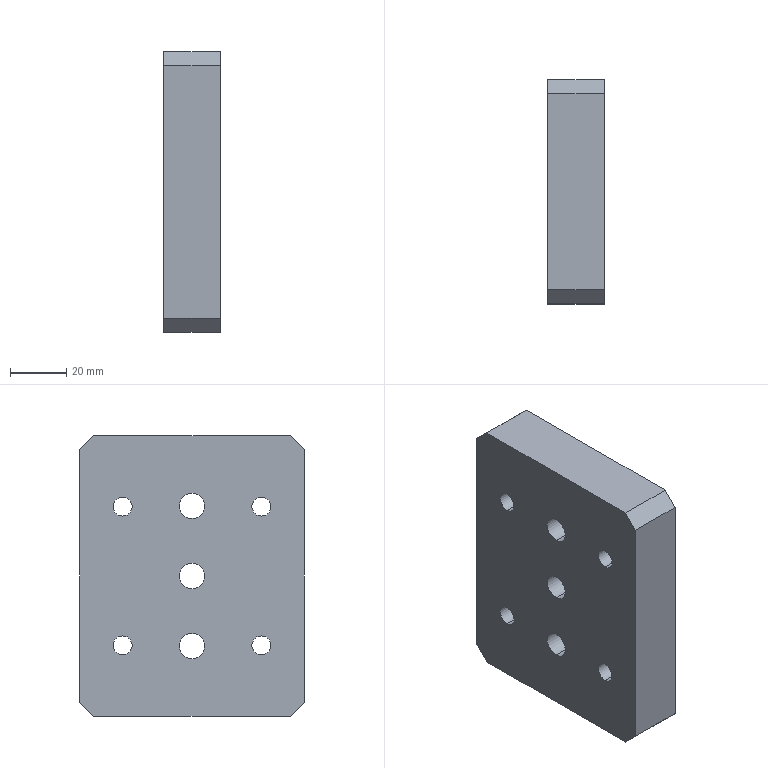Part | SolidWorks | features HoleWzd 2, Chamfer 1, Extrusion 1 | 1 solid | 33 faces | box 20 x 80 x 100 mm | volume 149224 mm3 | cylinder 20 | plane 13 | commonest cylinder face diameters 6.8 x8 9 x6 15 x6
STEP:
#1=CARTESIAN_POINT('',(11.,0.,32.5));
#2=VERTEX_POINT('',#1);
#3=CARTESIAN_POINT('',(11.,0.,17.5));
#4=VERTEX_POINT('',#3);
#5=CARTESIAN_POINT('',(11.,0.,25.));
#6=DIRECTION('',(1.,0.,0.));
#7=DIRECTION('',(0.,0.,-1.));
#8=AXIS2_PLACEMENT_3D('',#5,#6,#7);
#9=CIRCLE('',#8,7.5);
#10=EDGE_CURVE('',#2,#4,#9,.T.);
#11=ORIENTED_EDGE('',*,*,#10,.F.);
#12=CARTESIAN_POINT('',(20.,0.,32.5));
#13=VERTEX_POINT('',#12);
#14=CARTESIAN_POINT('',(20.,0.,32.5));
#15=DIRECTION('',(1.,0.,0.));
#16=VECTOR('',#15,1000.);
#17=LINE('',#14,#16);
#18=EDGE_CURVE('',#2,#13,#17,.T.);
#19=ORIENTED_EDGE('',*,*,#18,.T.);
#20=CARTESIAN_POINT('',(20.,0.,17.5));
#21=VERTEX_POINT('',#20);
#22=CARTESIAN_POINT('',(20.,0.,25.));
#23=DIRECTION('',(1.,0.,0.));
#24=DIRECTION('',(0.,0.,-1.));
#25=AXIS2_PLACEMENT_3D('',#22,#23,#24);
#26=CIRCLE('',#25,7.5);
#27=EDGE_CURVE('',#13,#21,#26,.T.);
#28=ORIENTED_EDGE('',*,*,#27,.T.);
#29=CARTESIAN_POINT('',(20.,0.,17.5));
#30=DIRECTION('',(1.,0.,0.));
#31=VECTOR('',#30,1000.);
#32=LINE('',#29,#31);
#33=EDGE_CURVE('',#4,#21,#32,.T.);
#34=ORIENTED_EDGE('',*,*,#33,.F.);
#35=EDGE_LOOP('',(#11,#19,#28,#34));
#36=FACE_OUTER_BOUND('',#35,.T.);
#37=CARTESIAN_POINT('',(20.,0.,25.));
#38=DIRECTION('',(1.,0.,0.));
#39=DIRECTION('',(0.,0.,-1.));
#40=AXIS2_PLACEMENT_3D('',#37,#38,#39);
#41=CYLINDRICAL_SURFACE('',#40,7.5);
#42=ADVANCED_FACE('',(#36),#41,.F.);
#43=CARTESIAN_POINT('',(0.,0.,29.5));
#44=VERTEX_POINT('',#43);
#45=CARTESIAN_POINT('',(0.,0.,20.5));
#46=VERTEX_POINT('',#45);
#47=CARTESIAN_POINT('',(0.,0.,25.));
#48=DIRECTION('',(1.,0.,0.));
#49=DIRECTION('',(0.,0.,-1.));
#50=AXIS2_PLACEMENT_3D('',#47,#48,#49);
#51=CIRCLE('',#50,4.5);
#52=EDGE_CURVE('',#44,#46,#51,.T.);
#53=ORIENTED_EDGE('',*,*,#52,.F.);
#54=CARTESIAN_POINT('',(11.,0.,29.5));
#55=VERTEX_POINT('',#54);
#56=CARTESIAN_POINT('',(20.,0.,29.5));
#57=DIRECTION('',(1.,0.,0.));
#58=VECTOR('',#57,1000.);
#59=LINE('',#56,#58);
#60=EDGE_CURVE('',#44,#55,#59,.T.);
#61=ORIENTED_EDGE('',*,*,#60,.T.);
#62=CARTESIAN_POINT('',(11.,0.,20.5));
#63=VERTEX_POINT('',#62);
#64=CARTESIAN_POINT('',(11.,0.,25.));
#65=DIRECTION('',(1.,0.,0.));
#66=DIRECTION('',(0.,0.,-1.));
#67=AXIS2_PLACEMENT_3D('',#64,#65,#66);
#68=CIRCLE('',#67,4.5);
#69=EDGE_CURVE('',#55,#63,#68,.T.);
#70=ORIENTED_EDGE('',*,*,#69,.T.);
#71=CARTESIAN_POINT('',(20.,0.,20.5));
#72=DIRECTION('',(1.,0.,0.));
#73=VECTOR('',#72,1000.);
#74=LINE('',#71,#73);
#75=EDGE_CURVE('',#46,#63,#74,.T.);
#76=ORIENTED_EDGE('',*,*,#75,.F.);
#77=EDGE_LOOP('',(#53,#61,#70,#76));
#78=FACE_OUTER_BOUND('',#77,.T.);
#79=CARTESIAN_POINT('',(20.,0.,25.));
#80=DIRECTION('',(1.,0.,0.));
#81=DIRECTION('',(0.,0.,-1.));
#82=AXIS2_PLACEMENT_3D('',#79,#80,#81);
#83=CYLINDRICAL_SURFACE('',#82,4.5);
#84=ADVANCED_FACE('',(#78),#83,.F.);
#85=CARTESIAN_POINT('',(11.,0.,7.5));
#86=VERTEX_POINT('',#85);
#87=CARTESIAN_POINT('',(11.,0.,-7.5));
#88=VERTEX_POINT('',#87);
#89=CARTESIAN_POINT('',(11.,0.,0.));
#90=DIRECTION('',(1.,0.,0.));
#91=DIRECTION('',(0.,0.,-1.));
#92=AXIS2_PLACEMENT_3D('',#89,#90,#91);
#93=CIRCLE('',#92,7.5);
#94=EDGE_CURVE('',#86,#88,#93,.T.);
#95=ORIENTED_EDGE('',*,*,#94,.F.);
#96=CARTESIAN_POINT('',(20.,0.,7.5));
#97=VERTEX_POINT('',#96);
#98=CARTESIAN_POINT('',(20.,0.,7.5));
#99=DIRECTION('',(1.,0.,0.));
#100=VECTOR('',#99,1000.);
#101=LINE('',#98,#100);
#102=EDGE_CURVE('',#86,#97,#101,.T.);
#103=ORIENTED_EDGE('',*,*,#102,.T.);
#104=CARTESIAN_POINT('',(20.,0.,-7.5));
#105=VERTEX_POINT('',#104);
#106=CARTESIAN_POINT('',(20.,0.,0.));
#107=DIRECTION('',(1.,0.,0.));
#108=DIRECTION('',(0.,0.,-1.));
#109=AXIS2_PLACEMENT_3D('',#106,#107,#108);
#110=CIRCLE('',#109,7.5);
#111=EDGE_CURVE('',#97,#105,#110,.T.);
#112=ORIENTED_EDGE('',*,*,#111,.T.);
#113=CARTESIAN_POINT('',(20.,0.,-7.5));
#114=DIRECTION('',(1.,0.,0.));
#115=VECTOR('',#114,1000.);
#116=LINE('',#113,#115);
#117=EDGE_CURVE('',#88,#105,#116,.T.);
#118=ORIENTED_EDGE('',*,*,#117,.F.);
#119=EDGE_LOOP('',(#95,#103,#112,#118));
#120=FACE_OUTER_BOUND('',#119,.T.);
#121=CARTESIAN_POINT('',(20.,0.,0.));
#122=DIRECTION('',(1.,0.,0.));
#123=DIRECTION('',(0.,0.,-1.));
#124=AXIS2_PLACEMENT_3D('',#121,#122,#123);
#125=CYLINDRICAL_SURFACE('',#124,7.5);
#126=ADVANCED_FACE('',(#120),#125,.F.);
#127=CARTESIAN_POINT('',(0.,0.,4.5));
#128=VERTEX_POINT('',#127);
#129=CARTESIAN_POINT('',(0.,0.,-4.5));
#130=VERTEX_POINT('',#129);
#131=CARTESIAN_POINT('',(0.,0.,0.));
#132=DIRECTION('',(1.,0.,0.));
#133=DIRECTION('',(0.,0.,-1.));
#134=AXIS2_PLACEMENT_3D('',#131,#132,#133);
#135=CIRCLE('',#134,4.5);
#136=EDGE_CURVE('',#128,#130,#135,.T.);
#137=ORIENTED_EDGE('',*,*,#136,.F.);
#138=CARTESIAN_POINT('',(11.,0.,4.5));
#139=VERTEX_POINT('',#138);
#140=CARTESIAN_POINT('',(20.,0.,4.5));
#141=DIRECTION('',(1.,0.,0.));
#142=VECTOR('',#141,1000.);
#143=LINE('',#140,#142);
#144=EDGE_CURVE('',#128,#139,#143,.T.);
#145=ORIENTED_EDGE('',*,*,#144,.T.);
#146=CARTESIAN_POINT('',(11.,0.,-4.5));
#147=VERTEX_POINT('',#146);
#148=CARTESIAN_POINT('',(11.,0.,0.));
#149=DIRECTION('',(1.,0.,0.));
#150=DIRECTION('',(0.,0.,-1.));
#151=AXIS2_PLACEMENT_3D('',#148,#149,#150);
#152=CIRCLE('',#151,4.5);
#153=EDGE_CURVE('',#139,#147,#152,.T.);
#154=ORIENTED_EDGE('',*,*,#153,.T.);
#155=CARTESIAN_POINT('',(20.,0.,-4.5));
#156=DIRECTION('',(1.,0.,0.));
#157=VECTOR('',#156,1000.);
#158=LINE('',#155,#157);
#159=EDGE_CURVE('',#130,#147,#158,.T.);
#160=ORIENTED_EDGE('',*,*,#159,.F.);
#161=EDGE_LOOP('',(#137,#145,#154,#160));
#162=FACE_OUTER_BOUND('',#161,.T.);
#163=CARTESIAN_POINT('',(20.,0.,0.));
#164=DIRECTION('',(1.,0.,0.));
#165=DIRECTION('',(0.,0.,-1.));
#166=AXIS2_PLACEMENT_3D('',#163,#164,#165);
#167=CYLINDRICAL_SURFACE('',#166,4.5);
#168=ADVANCED_FACE('',(#162),#167,.F.);
#169=CARTESIAN_POINT('',(11.,0.,-17.5));
#170=VERTEX_POINT('',#169);
#171=CARTESIAN_POINT('',(11.,0.,-32.5));
#172=VERTEX_POINT('',#171);
#173=CARTESIAN_POINT('',(11.,0.,-25.));
#174=DIRECTION('',(1.,0.,0.));
#175=DIRECTION('',(0.,0.,-1.));
#176=AXIS2_PLACEMENT_3D('',#173,#174,#175);
#177=CIRCLE('',#176,7.5);
#178=EDGE_CURVE('',#170,#172,#177,.T.);
#179=ORIENTED_EDGE('',*,*,#178,.F.);
#180=CARTESIAN_POINT('',(20.,0.,-17.5));
#181=VERTEX_POINT('',#180);
#182=CARTESIAN_POINT('',(20.,0.,-17.5));
#183=DIRECTION('',(1.,0.,0.));
#184=VECTOR('',#183,1000.);
#185=LINE('',#182,#184);
#186=EDGE_CURVE('',#170,#181,#185,.T.);
#187=ORIENTED_EDGE('',*,*,#186,.T.);
#188=CARTESIAN_POINT('',(20.,0.,-32.5));
#189=VERTEX_POINT('',#188);
#190=CARTESIAN_POINT('',(20.,0.,-25.));
#191=DIRECTION('',(1.,0.,0.));
#192=DIRECTION('',(0.,0.,-1.));
#193=AXIS2_PLACEMENT_3D('',#190,#191,#192);
#194=CIRCLE('',#193,7.5);
#195=EDGE_CURVE('',#181,#189,#194,.T.);
#196=ORIENTED_EDGE('',*,*,#195,.T.);
#197=CARTESIAN_POINT('',(20.,0.,-32.5));
#198=DIRECTION('',(1.,0.,0.));
#199=VECTOR('',#198,1000.);
#200=LINE('',#197,#199);
#201=EDGE_CURVE('',#172,#189,#200,.T.);
#202=ORIENTED_EDGE('',*,*,#201,.F.);
#203=EDGE_LOOP('',(#179,#187,#196,#202));
#204=FACE_OUTER_BOUND('',#203,.T.);
#205=CARTESIAN_POINT('',(20.,0.,-25.));
#206=DIRECTION('',(1.,0.,0.));
#207=DIRECTION('',(0.,0.,-1.));
#208=AXIS2_PLACEMENT_3D('',#205,#206,#207);
#209=CYLINDRICAL_SURFACE('',#208,7.5);
#210=ADVANCED_FACE('',(#204),#209,.F.);
#211=CARTESIAN_POINT('',(0.,0.,-20.5));
#212=VERTEX_POINT('',#211);
#213=CARTESIAN_POINT('',(0.,0.,-29.5));
#214=VERTEX_POINT('',#213);
#215=CARTESIAN_POINT('',(0.,0.,-25.));
#216=DIRECTION('',(1.,0.,0.));
#217=DIRECTION('',(0.,0.,-1.));
#218=AXIS2_PLACEMENT_3D('',#215,#216,#217);
#219=CIRCLE('',#218,4.5);
#220=EDGE_CURVE('',#212,#214,#219,.T.);
#221=ORIENTED_EDGE('',*,*,#220,.F.);
#222=CARTESIAN_POINT('',(11.,0.,-20.5));
#223=VERTEX_POINT('',#222);
#224=CARTESIAN_POINT('',(20.,0.,-20.5));
#225=DIRECTION('',(1.,0.,0.));
#226=VECTOR('',#225,1000.);
#227=LINE('',#224,#226);
#228=EDGE_CURVE('',#212,#223,#227,.T.);
#229=ORIENTED_EDGE('',*,*,#228,.T.);
#230=CARTESIAN_POINT('',(11.,0.,-29.5));
#231=VERTEX_POINT('',#230);
#232=CARTESIAN_POINT('',(11.,0.,-25.));
#233=DIRECTION('',(1.,0.,0.));
#234=DIRECTION('',(0.,0.,-1.));
#235=AXIS2_PLACEMENT_3D('',#232,#233,#234);
#236=CIRCLE('',#235,4.5);
#237=EDGE_CURVE('',#223,#231,#236,.T.);
#238=ORIENTED_EDGE('',*,*,#237,.T.);
#239=CARTESIAN_POINT('',(20.,0.,-29.5));
#240=DIRECTION('',(1.,0.,0.));
#241=VECTOR('',#240,1000.);
#242=LINE('',#239,#241);
#243=EDGE_CURVE('',#214,#231,#242,.T.);
#244=ORIENTED_EDGE('',*,*,#243,.F.);
#245=EDGE_LOOP('',(#221,#229,#238,#244));
#246=FACE_OUTER_BOUND('',#245,.T.);
#247=CARTESIAN_POINT('',(20.,0.,-25.));
#248=DIRECTION('',(1.,0.,0.));
#249=DIRECTION('',(0.,0.,-1.));
#250=AXIS2_PLACEMENT_3D('',#247,#248,#249);
#251=CYLINDRICAL_SURFACE('',#250,4.5);
#252=ADVANCED_FACE('',(#246),#251,.F.);
#253=CARTESIAN_POINT('',(0.,24.749,28.149));
#254=VERTEX_POINT('',#253);
#255=CARTESIAN_POINT('',(0.,24.749,21.349));
#256=VERTEX_POINT('',#255);
#257=CARTESIAN_POINT('',(0.,24.749,24.749));
#258=DIRECTION('',(1.,0.,0.));
#259=DIRECTION('',(0.,0.,-1.));
#260=AXIS2_PLACEMENT_3D('',#257,#258,#259);
#261=CIRCLE('',#260,3.4);
#262=EDGE_CURVE('',#254,#256,#261,.T.);
#263=ORIENTED_EDGE('',*,*,#262,.F.);
#264=CARTESIAN_POINT('',(20.,24.749,28.149));
#265=VERTEX_POINT('',#264);
#266=CARTESIAN_POINT('',(20.,24.749,28.149));
#267=DIRECTION('',(1.,0.,0.));
#268=VECTOR('',#267,1000.);
#269=LINE('',#266,#268);
#270=EDGE_CURVE('',#254,#265,#269,.T.);
#271=ORIENTED_EDGE('',*,*,#270,.T.);
#272=CARTESIAN_POINT('',(20.,24.749,21.349));
#273=VERTEX_POINT('',#272);
#274=CARTESIAN_POINT('',(20.,24.749,24.749));
#275=DIRECTION('',(1.,0.,0.));
#276=DIRECTION('',(0.,0.,-1.));
#277=AXIS2_PLACEMENT_3D('',#274,#275,#276);
#278=CIRCLE('',#277,3.4);
#279=EDGE_CURVE('',#265,#273,#278,.T.);
#280=ORIENTED_EDGE('',*,*,#279,.T.);
#281=CARTESIAN_POINT('',(20.,24.749,21.349));
#282=DIRECTION('',(1.,0.,0.));
#283=VECTOR('',#282,1000.);
#284=LINE('',#281,#283);
#285=EDGE_CURVE('',#256,#273,#284,.T.);
#286=ORIENTED_EDGE('',*,*,#285,.F.);
#287=EDGE_LOOP('',(#263,#271,#280,#286));
#288=FACE_OUTER_BOUND('',#287,.T.);
#289=CARTESIAN_POINT('',(20.,24.749,24.749));
#290=DIRECTION('',(1.,0.,0.));
#291=DIRECTION('',(0.,0.,-1.));
#292=AXIS2_PLACEMENT_3D('',#289,#290,#291);
#293=CYLINDRICAL_SURFACE('',#292,3.4);
#294=ADVANCED_FACE('',(#288),#293,.F.);
#295=CARTESIAN_POINT('',(0.,24.749,-21.349));
#296=VERTEX_POINT('',#295);
#297=CARTESIAN_POINT('',(0.,24.749,-28.149));
#298=VERTEX_POINT('',#297);
#299=CARTESIAN_POINT('',(0.,24.749,-24.749));
#300=DIRECTION('',(1.,0.,0.));
#301=DIRECTION('',(0.,0.,-1.));
#302=AXIS2_PLACEMENT_3D('',#299,#300,#301);
#303=CIRCLE('',#302,3.4);
#304=EDGE_CURVE('',#296,#298,#303,.T.);
#305=ORIENTED_EDGE('',*,*,#304,.F.);
#306=CARTESIAN_POINT('',(20.,24.749,-21.349));
#307=VERTEX_POINT('',#306);
#308=CARTESIAN_POINT('',(20.,24.749,-21.349));
#309=DIRECTION('',(1.,0.,0.));
#310=VECTOR('',#309,1000.);
#311=LINE('',#308,#310);
#312=EDGE_CURVE('',#296,#307,#311,.T.);
#313=ORIENTED_EDGE('',*,*,#312,.T.);
#314=CARTESIAN_POINT('',(20.,24.749,-28.149));
#315=VERTEX_POINT('',#314);
#316=CARTESIAN_POINT('',(20.,24.749,-24.749));
#317=DIRECTION('',(1.,0.,0.));
#318=DIRECTION('',(0.,0.,-1.));
#319=AXIS2_PLACEMENT_3D('',#316,#317,#318);
#320=CIRCLE('',#319,3.4);
#321=EDGE_CURVE('',#307,#315,#320,.T.);
#322=ORIENTED_EDGE('',*,*,#321,.T.);
#323=CARTESIAN_POINT('',(20.,24.749,-28.149));
#324=DIRECTION('',(1.,0.,0.));
#325=VECTOR('',#324,1000.);
#326=LINE('',#323,#325);
#327=EDGE_CURVE('',#298,#315,#326,.T.);
#328=ORIENTED_EDGE('',*,*,#327,.F.);
#329=EDGE_LOOP('',(#305,#313,#322,#328));
#330=FACE_OUTER_BOUND('',#329,.T.);
#331=CARTESIAN_POINT('',(20.,24.749,-24.749));
#332=DIRECTION('',(1.,0.,0.));
#333=DIRECTION('',(0.,0.,-1.));
#334=AXIS2_PLACEMENT_3D('',#331,#332,#333);
#335=CYLINDRICAL_SURFACE('',#334,3.4);
#336=ADVANCED_FACE('',(#330),#335,.F.);
#337=CARTESIAN_POINT('',(0.,-24.749,-21.349));
#338=VERTEX_POINT('',#337);
#339=CARTESIAN_POINT('',(0.,-24.749,-28.149));
#340=VERTEX_POINT('',#339);
#341=CARTESIAN_POINT('',(0.,-24.749,-24.749));
#342=DIRECTION('',(1.,0.,0.));
#343=DIRECTION('',(0.,0.,-1.));
#344=AXIS2_PLACEMENT_3D('',#341,#342,#343);
#345=CIRCLE('',#344,3.4);
#346=EDGE_CURVE('',#338,#340,#345,.T.);
#347=ORIENTED_EDGE('',*,*,#346,.F.);
#348=CARTESIAN_POINT('',(20.,-24.749,-21.349));
#349=VERTEX_POINT('',#348);
#350=CARTESIAN_POINT('',(20.,-24.749,-21.349));
#351=DIRECTION('',(1.,0.,0.));
#352=VECTOR('',#351,1000.);
#353=LINE('',#350,#352);
#354=EDGE_CURVE('',#338,#349,#353,.T.);
#355=ORIENTED_EDGE('',*,*,#354,.T.);
#356=CARTESIAN_POINT('',(20.,-24.749,-28.149));
#357=VERTEX_POINT('',#356);
#358=CARTESIAN_POINT('',(20.,-24.749,-24.749));
#359=DIRECTION('',(1.,0.,0.));
#360=DIRECTION('',(0.,0.,-1.));
#361=AXIS2_PLACEMENT_3D('',#358,#359,#360);
#362=CIRCLE('',#361,3.4);
#363=EDGE_CURVE('',#349,#357,#362,.T.);
#364=ORIENTED_EDGE('',*,*,#363,.T.);
#365=CARTESIAN_POINT('',(20.,-24.749,-28.149));
#366=DIRECTION('',(1.,0.,0.));
#367=VECTOR('',#366,1000.);
#368=LINE('',#365,#367);
#369=EDGE_CURVE('',#340,#357,#368,.T.);
#370=ORIENTED_EDGE('',*,*,#369,.F.);
#371=EDGE_LOOP('',(#347,#355,#364,#370));
#372=FACE_OUTER_BOUND('',#371,.T.);
#373=CARTESIAN_POINT('',(20.,-24.749,-24.749));
#374=DIRECTION('',(1.,0.,0.));
#375=DIRECTION('',(0.,0.,-1.));
#376=AXIS2_PLACEMENT_3D('',#373,#374,#375);
#377=CYLINDRICAL_SURFACE('',#376,3.4);
#378=ADVANCED_FACE('',(#372),#377,.F.);
#379=CARTESIAN_POINT('',(0.,-24.749,28.149));
#380=VERTEX_POINT('',#379);
#381=CARTESIAN_POINT('',(0.,-24.749,21.349));
#382=VERTEX_POINT('',#381);
#383=CARTESIAN_POINT('',(0.,-24.749,24.749));
#384=DIRECTION('',(1.,0.,0.));
#385=DIRECTION('',(0.,0.,-1.));
#386=AXIS2_PLACEMENT_3D('',#383,#384,#385);
#387=CIRCLE('',#386,3.4);
#388=EDGE_CURVE('',#380,#382,#387,.T.);
#389=ORIENTED_EDGE('',*,*,#388,.F.);
#390=CARTESIAN_POINT('',(20.,-24.749,28.149));
#391=VERTEX_POINT('',#390);
#392=CARTESIAN_POINT('',(20.,-24.749,28.149));
#393=DIRECTION('',(1.,0.,0.));
#394=VECTOR('',#393,1000.);
#395=LINE('',#392,#394);
#396=EDGE_CURVE('',#380,#391,#395,.T.);
#397=ORIENTED_EDGE('',*,*,#396,.T.);
#398=CARTESIAN_POINT('',(20.,-24.749,21.349));
#399=VERTEX_POINT('',#398);
#400=CARTESIAN_POINT('',(20.,-24.749,24.749));
#401=DIRECTION('',(1.,0.,0.));
#402=DIRECTION('',(0.,0.,-1.));
#403=AXIS2_PLACEMENT_3D('',#400,#401,#402);
#404=CIRCLE('',#403,3.4);
#405=EDGE_CURVE('',#391,#399,#404,.T.);
#406=ORIENTED_EDGE('',*,*,#405,.T.);
#407=CARTESIAN_POINT('',(20.,-24.749,21.349));
#408=DIRECTION('',(1.,0.,0.));
#409=VECTOR('',#408,1000.);
#410=LINE('',#407,#409);
#411=EDGE_CURVE('',#382,#399,#410,.T.);
#412=ORIENTED_EDGE('',*,*,#411,.F.);
#413=EDGE_LOOP('',(#389,#397,#406,#412));
#414=FACE_OUTER_BOUND('',#413,.T.);
#415=CARTESIAN_POINT('',(20.,-24.749,24.749));
#416=DIRECTION('',(1.,0.,0.));
#417=DIRECTION('',(0.,0.,-1.));
#418=AXIS2_PLACEMENT_3D('',#415,#416,#417);
#419=CYLINDRICAL_SURFACE('',#418,3.4);
#420=ADVANCED_FACE('',(#414),#419,.F.);
#421=CARTESIAN_POINT('',(0.,-35.,-50.));
#422=VERTEX_POINT('',#421);
#423=CARTESIAN_POINT('',(0.,35.,-50.));
#424=VERTEX_POINT('',#423);
#425=CARTESIAN_POINT('',(0.,40.,-50.));
#426=DIRECTION('',(0.,1.,0.));
#427=VECTOR('',#426,1000.);
#428=LINE('',#425,#427);
#429=EDGE_CURVE('',#422,#424,#428,.T.);
#430=ORIENTED_EDGE('',*,*,#429,.T.);
#431=CARTESIAN_POINT('',(20.,35.,-50.));
#432=VERTEX_POINT('',#431);
#433=CARTESIAN_POINT('',(20.,35.,-50.));
#434=DIRECTION('',(1.,0.,0.));
#435=VECTOR('',#434,1000.);
#436=LINE('',#433,#435);
#437=EDGE_CURVE('',#424,#432,#436,.T.);
#438=ORIENTED_EDGE('',*,*,#437,.T.);
#439=CARTESIAN_POINT('',(20.,-35.,-50.));
#440=VERTEX_POINT('',#439);
#441=CARTESIAN_POINT('',(20.,40.,-50.));
#442=DIRECTION('',(0.,1.,0.));
#443=VECTOR('',#442,1000.);
#444=LINE('',#441,#443);
#445=EDGE_CURVE('',#440,#432,#444,.T.);
#446=ORIENTED_EDGE('',*,*,#445,.F.);
#447=CARTESIAN_POINT('',(20.,-35.,-50.));
#448=DIRECTION('',(-1.,0.,0.));
#449=VECTOR('',#448,1000.);
#450=LINE('',#447,#449);
#451=EDGE_CURVE('',#440,#422,#450,.T.);
#452=ORIENTED_EDGE('',*,*,#451,.T.);
#453=EDGE_LOOP('',(#430,#438,#446,#452));
#454=FACE_OUTER_BOUND('',#453,.T.);
#455=CARTESIAN_POINT('',(20.,40.,-50.));
#456=DIRECTION('',(0.,0.,1.));
#457=DIRECTION('',(0.,-1.,0.));
#458=AXIS2_PLACEMENT_3D('',#455,#456,#457);
#459=PLANE('',#458);
#460=ADVANCED_FACE('',(#454),#459,.F.);
#461=CARTESIAN_POINT('',(20.,40.,-45.));
#462=VERTEX_POINT('',#461);
#463=CARTESIAN_POINT('',(20.,40.,45.));
#464=VERTEX_POINT('',#463);
#465=CARTESIAN_POINT('',(20.,40.,50.));
#466=DIRECTION('',(0.,0.,1.));
#467=VECTOR('',#466,1000.);
#468=LINE('',#465,#467);
#469=EDGE_CURVE('',#462,#464,#468,.T.);
#470=ORIENTED_EDGE('',*,*,#469,.F.);
#471=CARTESIAN_POINT('',(0.,40.,-45.));
#472=VERTEX_POINT('',#471);
#473=CARTESIAN_POINT('',(20.,40.,-45.));
#474=DIRECTION('',(-1.,0.,0.));
#475=VECTOR('',#474,1000.);
#476=LINE('',#473,#475);
#477=EDGE_CURVE('',#462,#472,#476,.T.);
#478=ORIENTED_EDGE('',*,*,#477,.T.);
#479=CARTESIAN_POINT('',(0.,40.,45.));
#480=VERTEX_POINT('',#479);
#481=CARTESIAN_POINT('',(0.,40.,50.));
#482=DIRECTION('',(0.,0.,1.));
#483=VECTOR('',#482,1000.);
#484=LINE('',#481,#483);
#485=EDGE_CURVE('',#472,#480,#484,.T.);
#486=ORIENTED_EDGE('',*,*,#485,.T.);
#487=CARTESIAN_POINT('',(20.,40.,45.));
#488=DIRECTION('',(1.,0.,0.));
#489=VECTOR('',#488,1000.);
#490=LINE('',#487,#489);
#491=EDGE_CURVE('',#480,#464,#490,.T.);
#492=ORIENTED_EDGE('',*,*,#491,.T.);
#493=EDGE_LOOP('',(#470,#478,#486,#492));
#494=FACE_OUTER_BOUND('',#493,.T.);
#495=CARTESIAN_POINT('',(20.,40.,50.));
#496=DIRECTION('',(0.,-1.,0.));
#497=DIRECTION('',(0.,0.,-1.));
#498=AXIS2_PLACEMENT_3D('',#495,#496,#497);
#499=PLANE('',#498);
#500=ADVANCED_FACE('',(#494),#499,.F.);
#501=CARTESIAN_POINT('',(20.,35.,50.));
#502=VERTEX_POINT('',#501);
#503=CARTESIAN_POINT('',(20.,-35.,50.));
#504=VERTEX_POINT('',#503);
#505=CARTESIAN_POINT('',(20.,40.,50.));
#506=DIRECTION('',(0.,-1.,0.));
#507=VECTOR('',#506,1000.);
#508=LINE('',#505,#507);
#509=EDGE_CURVE('',#502,#504,#508,.T.);
#510=ORIENTED_EDGE('',*,*,#509,.F.);
#511=CARTESIAN_POINT('',(0.,35.,50.));
#512=VERTEX_POINT('',#511);
#513=CARTESIAN_POINT('',(20.,35.,50.));
#514=DIRECTION('',(-1.,0.,0.));
#515=VECTOR('',#514,1000.);
#516=LINE('',#513,#515);
#517=EDGE_CURVE('',#502,#512,#516,.T.);
#518=ORIENTED_EDGE('',*,*,#517,.T.);
#519=CARTESIAN_POINT('',(0.,-35.,50.));
#520=VERTEX_POINT('',#519);
#521=CARTESIAN_POINT('',(0.,40.,50.));
#522=DIRECTION('',(0.,-1.,0.));
#523=VECTOR('',#522,1000.);
#524=LINE('',#521,#523);
#525=EDGE_CURVE('',#512,#520,#524,.T.);
#526=ORIENTED_EDGE('',*,*,#525,.T.);
#527=CARTESIAN_POINT('',(20.,-35.,50.));
#528=DIRECTION('',(1.,0.,0.));
#529=VECTOR('',#528,1000.);
#530=LINE('',#527,#529);
#531=EDGE_CURVE('',#520,#504,#530,.T.);
#532=ORIENTED_EDGE('',*,*,#531,.T.);
#533=EDGE_LOOP('',(#510,#518,#526,#532));
#534=FACE_OUTER_BOUND('',#533,.T.);
#535=CARTESIAN_POINT('',(20.,40.,50.));
#536=DIRECTION('',(0.,0.,-1.));
#537=DIRECTION('',(0.,1.,0.));
#538=AXIS2_PLACEMENT_3D('',#535,#536,#537);
#539=PLANE('',#538);
#540=ADVANCED_FACE('',(#534),#539,.F.);
#541=CARTESIAN_POINT('',(0.,-40.,45.));
#542=VERTEX_POINT('',#541);
#543=CARTESIAN_POINT('',(0.,-40.,-45.));
#544=VERTEX_POINT('',#543);
#545=CARTESIAN_POINT('',(0.,-40.,50.));
#546=DIRECTION('',(0.,0.,-1.));
#547=VECTOR('',#546,1000.);
#548=LINE('',#545,#547);
#549=EDGE_CURVE('',#542,#544,#548,.T.);
#550=ORIENTED_EDGE('',*,*,#549,.T.);
#551=CARTESIAN_POINT('',(20.,-40.,-45.));
#552=VERTEX_POINT('',#551);
#553=CARTESIAN_POINT('',(20.,-40.,-45.));
#554=DIRECTION('',(1.,0.,0.));
#555=VECTOR('',#554,1000.);
#556=LINE('',#553,#555);
#557=EDGE_CURVE('',#544,#552,#556,.T.);
#558=ORIENTED_EDGE('',*,*,#557,.T.);
#559=CARTESIAN_POINT('',(20.,-40.,45.));
#560=VERTEX_POINT('',#559);
#561=CARTESIAN_POINT('',(20.,-40.,50.));
#562=DIRECTION('',(0.,0.,-1.));
#563=VECTOR('',#562,1000.);
#564=LINE('',#561,#563);
#565=EDGE_CURVE('',#560,#552,#564,.T.);
#566=ORIENTED_EDGE('',*,*,#565,.F.);
#567=CARTESIAN_POINT('',(20.,-40.,45.));
#568=DIRECTION('',(-1.,0.,0.));
#569=VECTOR('',#568,1000.);
#570=LINE('',#567,#569);
#571=EDGE_CURVE('',#560,#542,#570,.T.);
#572=ORIENTED_EDGE('',*,*,#571,.T.);
#573=EDGE_LOOP('',(#550,#558,#566,#572));
#574=FACE_OUTER_BOUND('',#573,.T.);
#575=CARTESIAN_POINT('',(20.,-40.,50.));
#576=DIRECTION('',(0.,1.,0.));
#577=DIRECTION('',(0.,0.,1.));
#578=AXIS2_PLACEMENT_3D('',#575,#576,#577);
#579=PLANE('',#578);
#580=ADVANCED_FACE('',(#574),#579,.F.);
#581=CARTESIAN_POINT('',(20.,0.,25.));
#582=DIRECTION('',(1.,0.,0.));
#583=DIRECTION('',(0.,0.,-1.));
#584=AXIS2_PLACEMENT_3D('',#581,#582,#583);
#585=CIRCLE('',#584,7.5);
#586=EDGE_CURVE('',#21,#13,#585,.T.);
#587=ORIENTED_EDGE('',*,*,#586,.F.);
#588=ORIENTED_EDGE('',*,*,#27,.F.);
#589=EDGE_LOOP('',(#587,#588));
#590=FACE_BOUND('',#589,.T.);
#591=CARTESIAN_POINT('',(20.,0.,0.));
#592=DIRECTION('',(1.,0.,0.));
#593=DIRECTION('',(0.,0.,-1.));
#594=AXIS2_PLACEMENT_3D('',#591,#592,#593);
#595=CIRCLE('',#594,7.5);
#596=EDGE_CURVE('',#105,#97,#595,.T.);
#597=ORIENTED_EDGE('',*,*,#596,.F.);
#598=ORIENTED_EDGE('',*,*,#111,.F.);
#599=EDGE_LOOP('',(#597,#598));
#600=FACE_BOUND('',#599,.T.);
#601=CARTESIAN_POINT('',(20.,0.,-25.));
#602=DIRECTION('',(1.,0.,0.));
#603=DIRECTION('',(0.,0.,-1.));
#604=AXIS2_PLACEMENT_3D('',#601,#602,#603);
#605=CIRCLE('',#604,7.5);
#606=EDGE_CURVE('',#189,#181,#605,.T.);
#607=ORIENTED_EDGE('',*,*,#606,.F.);
#608=ORIENTED_EDGE('',*,*,#195,.F.);
#609=EDGE_LOOP('',(#607,#608));
#610=FACE_BOUND('',#609,.T.);
#611=CARTESIAN_POINT('',(20.,24.749,24.749));
#612=DIRECTION('',(1.,0.,0.));
#613=DIRECTION('',(0.,0.,-1.));
#614=AXIS2_PLACEMENT_3D('',#611,#612,#613);
#615=CIRCLE('',#614,3.4);
#616=EDGE_CURVE('',#273,#265,#615,.T.);
#617=ORIENTED_EDGE('',*,*,#616,.F.);
#618=ORIENTED_EDGE('',*,*,#279,.F.);
#619=EDGE_LOOP('',(#617,#618));
#620=FACE_BOUND('',#619,.T.);
#621=CARTESIAN_POINT('',(20.,24.749,-24.749));
#622=DIRECTION('',(1.,0.,0.));
#623=DIRECTION('',(0.,0.,-1.));
#624=AXIS2_PLACEMENT_3D('',#621,#622,#623);
#625=CIRCLE('',#624,3.4);
#626=EDGE_CURVE('',#315,#307,#625,.T.);
#627=ORIENTED_EDGE('',*,*,#626,.F.);
#628=ORIENTED_EDGE('',*,*,#321,.F.);
#629=EDGE_LOOP('',(#627,#628));
#630=FACE_BOUND('',#629,.T.);
#631=CARTESIAN_POINT('',(20.,-24.749,-24.749));
#632=DIRECTION('',(1.,0.,0.));
#633=DIRECTION('',(0.,0.,-1.));
#634=AXIS2_PLACEMENT_3D('',#631,#632,#633);
#635=CIRCLE('',#634,3.4);
#636=EDGE_CURVE('',#357,#349,#635,.T.);
#637=ORIENTED_EDGE('',*,*,#636,.F.);
#638=ORIENTED_EDGE('',*,*,#363,.F.);
#639=EDGE_LOOP('',(#637,#638));
#640=FACE_BOUND('',#639,.T.);
#641=CARTESIAN_POINT('',(20.,-24.749,24.749));
#642=DIRECTION('',(1.,0.,0.));
#643=DIRECTION('',(0.,0.,-1.));
#644=AXIS2_PLACEMENT_3D('',#641,#642,#643);
#645=CIRCLE('',#644,3.4);
#646=EDGE_CURVE('',#399,#391,#645,.T.);
#647=ORIENTED_EDGE('',*,*,#646,.F.);
#648=ORIENTED_EDGE('',*,*,#405,.F.);
#649=EDGE_LOOP('',(#647,#648));
#650=FACE_BOUND('',#649,.T.);
#651=ORIENTED_EDGE('',*,*,#445,.T.);
#652=CARTESIAN_POINT('',(20.,42.5,-42.5));
#653=DIRECTION('',(0.,0.7071,0.7071));
#654=VECTOR('',#653,1000.);
#655=LINE('',#652,#654);
#656=EDGE_CURVE('',#432,#462,#655,.T.);
#657=ORIENTED_EDGE('',*,*,#656,.T.);
#658=ORIENTED_EDGE('',*,*,#469,.T.);
#659=CARTESIAN_POINT('',(20.,42.5,42.5));
#660=DIRECTION('',(0.,-0.7071,0.7071));
#661=VECTOR('',#660,1000.);
#662=LINE('',#659,#661);
#663=EDGE_CURVE('',#464,#502,#662,.T.);
#664=ORIENTED_EDGE('',*,*,#663,.T.);
#665=ORIENTED_EDGE('',*,*,#509,.T.);
#666=CARTESIAN_POINT('',(20.,-42.5,42.5));
#667=DIRECTION('',(0.,-0.7071,-0.7071));
#668=VECTOR('',#667,1000.);
#669=LINE('',#666,#668);
#670=EDGE_CURVE('',#504,#560,#669,.T.);
#671=ORIENTED_EDGE('',*,*,#670,.T.);
#672=ORIENTED_EDGE('',*,*,#565,.T.);
#673=CARTESIAN_POINT('',(20.,-42.5,-42.5));
#674=DIRECTION('',(0.,0.7071,-0.7071));
#675=VECTOR('',#674,1000.);
#676=LINE('',#673,#675);
#677=EDGE_CURVE('',#552,#440,#676,.T.);
#678=ORIENTED_EDGE('',*,*,#677,.T.);
#679=EDGE_LOOP('',(#651,#657,#658,#664,#665,#671,#672,#678));
#680=FACE_OUTER_BOUND('',#679,.T.);
#681=CARTESIAN_POINT('',(20.,0.,0.));
#682=DIRECTION('',(1.,0.,0.));
#683=DIRECTION('',(0.,0.,-1.));
#684=AXIS2_PLACEMENT_3D('',#681,#682,#683);
#685=PLANE('',#684);
#686=ADVANCED_FACE('',(#590,#600,#610,#620,#630,#640,#650,#680),#685,.T.);
#687=CARTESIAN_POINT('',(0.,0.,25.));
#688=DIRECTION('',(1.,0.,0.));
#689=DIRECTION('',(0.,0.,-1.));
#690=AXIS2_PLACEMENT_3D('',#687,#688,#689);
#691=CIRCLE('',#690,4.5);
#692=EDGE_CURVE('',#46,#44,#691,.T.);
#693=ORIENTED_EDGE('',*,*,#692,.T.);
#694=ORIENTED_EDGE('',*,*,#52,.T.);
#695=EDGE_LOOP('',(#693,#694));
#696=FACE_BOUND('',#695,.T.);
#697=CARTESIAN_POINT('',(0.,0.,0.));
#698=DIRECTION('',(1.,0.,0.));
#699=DIRECTION('',(0.,0.,-1.));
#700=AXIS2_PLACEMENT_3D('',#697,#698,#699);
#701=CIRCLE('',#700,4.5);
#702=EDGE_CURVE('',#130,#128,#701,.T.);
#703=ORIENTED_EDGE('',*,*,#702,.T.);
#704=ORIENTED_EDGE('',*,*,#136,.T.);
#705=EDGE_LOOP('',(#703,#704));
#706=FACE_BOUND('',#705,.T.);
#707=CARTESIAN_POINT('',(0.,0.,-25.));
#708=DIRECTION('',(1.,0.,0.));
#709=DIRECTION('',(0.,0.,-1.));
#710=AXIS2_PLACEMENT_3D('',#707,#708,#709);
#711=CIRCLE('',#710,4.5);
#712=EDGE_CURVE('',#214,#212,#711,.T.);
#713=ORIENTED_EDGE('',*,*,#712,.T.);
#714=ORIENTED_EDGE('',*,*,#220,.T.);
#715=EDGE_LOOP('',(#713,#714));
#716=FACE_BOUND('',#715,.T.);
#717=CARTESIAN_POINT('',(0.,24.749,24.749));
#718=DIRECTION('',(1.,0.,0.));
#719=DIRECTION('',(0.,0.,-1.));
#720=AXIS2_PLACEMENT_3D('',#717,#718,#719);
#721=CIRCLE('',#720,3.4);
#722=EDGE_CURVE('',#256,#254,#721,.T.);
#723=ORIENTED_EDGE('',*,*,#722,.T.);
#724=ORIENTED_EDGE('',*,*,#262,.T.);
#725=EDGE_LOOP('',(#723,#724));
#726=FACE_BOUND('',#725,.T.);
#727=CARTESIAN_POINT('',(0.,24.749,-24.749));
#728=DIRECTION('',(1.,0.,0.));
#729=DIRECTION('',(0.,0.,-1.));
#730=AXIS2_PLACEMENT_3D('',#727,#728,#729);
#731=CIRCLE('',#730,3.4);
#732=EDGE_CURVE('',#298,#296,#731,.T.);
#733=ORIENTED_EDGE('',*,*,#732,.T.);
#734=ORIENTED_EDGE('',*,*,#304,.T.);
#735=EDGE_LOOP('',(#733,#734));
#736=FACE_BOUND('',#735,.T.);
#737=CARTESIAN_POINT('',(0.,-24.749,-24.749));
#738=DIRECTION('',(1.,0.,0.));
#739=DIRECTION('',(0.,0.,-1.));
#740=AXIS2_PLACEMENT_3D('',#737,#738,#739);
#741=CIRCLE('',#740,3.4);
#742=EDGE_CURVE('',#340,#338,#741,.T.);
#743=ORIENTED_EDGE('',*,*,#742,.T.);
#744=ORIENTED_EDGE('',*,*,#346,.T.);
#745=EDGE_LOOP('',(#743,#744));
#746=FACE_BOUND('',#745,.T.);
#747=CARTESIAN_POINT('',(0.,-24.749,24.749));
#748=DIRECTION('',(1.,0.,0.));
#749=DIRECTION('',(0.,0.,-1.));
#750=AXIS2_PLACEMENT_3D('',#747,#748,#749);
#751=CIRCLE('',#750,3.4);
#752=EDGE_CURVE('',#382,#380,#751,.T.);
#753=ORIENTED_EDGE('',*,*,#752,.T.);
#754=ORIENTED_EDGE('',*,*,#388,.T.);
#755=EDGE_LOOP('',(#753,#754));
#756=FACE_BOUND('',#755,.T.);
#757=ORIENTED_EDGE('',*,*,#485,.F.);
#758=CARTESIAN_POINT('',(0.,40.,-45.));
#759=DIRECTION('',(0.,-0.7071,-0.7071));
#760=VECTOR('',#759,1000.);
#761=LINE('',#758,#760);
#762=EDGE_CURVE('',#472,#424,#761,.T.);
#763=ORIENTED_EDGE('',*,*,#762,.T.);
#764=ORIENTED_EDGE('',*,*,#429,.F.);
#765=CARTESIAN_POINT('',(0.,-35.,-50.));
#766=DIRECTION('',(0.,-0.7071,0.7071));
#767=VECTOR('',#766,1000.);
#768=LINE('',#765,#767);
#769=EDGE_CURVE('',#422,#544,#768,.T.);
#770=ORIENTED_EDGE('',*,*,#769,.T.);
#771=ORIENTED_EDGE('',*,*,#549,.F.);
#772=CARTESIAN_POINT('',(0.,-40.,45.));
#773=DIRECTION('',(0.,0.7071,0.7071));
#774=VECTOR('',#773,1000.);
#775=LINE('',#772,#774);
#776=EDGE_CURVE('',#542,#520,#775,.T.);
#777=ORIENTED_EDGE('',*,*,#776,.T.);
#778=ORIENTED_EDGE('',*,*,#525,.F.);
#779=CARTESIAN_POINT('',(0.,35.,50.));
#780=DIRECTION('',(0.,0.7071,-0.7071));
#781=VECTOR('',#780,1000.);
#782=LINE('',#779,#781);
#783=EDGE_CURVE('',#512,#480,#782,.T.);
#784=ORIENTED_EDGE('',*,*,#783,.T.);
#785=EDGE_LOOP('',(#757,#763,#764,#770,#771,#777,#778,#784));
#786=FACE_OUTER_BOUND('',#785,.T.);
#787=CARTESIAN_POINT('',(0.,0.,0.));
#788=DIRECTION('',(1.,0.,0.));
#789=DIRECTION('',(0.,0.,-1.));
#790=AXIS2_PLACEMENT_3D('',#787,#788,#789);
#791=PLANE('',#790);
#792=ADVANCED_FACE('',(#696,#706,#716,#726,#736,#746,#756,#786),#791,.F.);
#793=ORIENTED_EDGE('',*,*,#396,.F.);
#794=ORIENTED_EDGE('',*,*,#752,.F.);
#795=ORIENTED_EDGE('',*,*,#411,.T.);
#796=ORIENTED_EDGE('',*,*,#646,.T.);
#797=EDGE_LOOP('',(#793,#794,#795,#796));
#798=FACE_OUTER_BOUND('',#797,.T.);
#799=CARTESIAN_POINT('',(20.,-24.749,24.749));
#800=DIRECTION('',(1.,0.,0.));
#801=DIRECTION('',(0.,0.,-1.));
#802=AXIS2_PLACEMENT_3D('',#799,#800,#801);
#803=CYLINDRICAL_SURFACE('',#802,3.4);
#804=ADVANCED_FACE('',(#798),#803,.F.);
#805=ORIENTED_EDGE('',*,*,#354,.F.);
#806=ORIENTED_EDGE('',*,*,#742,.F.);
#807=ORIENTED_EDGE('',*,*,#369,.T.);
#808=ORIENTED_EDGE('',*,*,#636,.T.);
#809=EDGE_LOOP('',(#805,#806,#807,#808));
#810=FACE_OUTER_BOUND('',#809,.T.);
#811=CARTESIAN_POINT('',(20.,-24.749,-24.749));
#812=DIRECTION('',(1.,0.,0.));
#813=DIRECTION('',(0.,0.,-1.));
#814=AXIS2_PLACEMENT_3D('',#811,#812,#813);
#815=CYLINDRICAL_SURFACE('',#814,3.4);
#816=ADVANCED_FACE('',(#810),#815,.F.);
#817=ORIENTED_EDGE('',*,*,#312,.F.);
#818=ORIENTED_EDGE('',*,*,#732,.F.);
#819=ORIENTED_EDGE('',*,*,#327,.T.);
#820=ORIENTED_EDGE('',*,*,#626,.T.);
#821=EDGE_LOOP('',(#817,#818,#819,#820));
#822=FACE_OUTER_BOUND('',#821,.T.);
#823=CARTESIAN_POINT('',(20.,24.749,-24.749));
#824=DIRECTION('',(1.,0.,0.));
#825=DIRECTION('',(0.,0.,-1.));
#826=AXIS2_PLACEMENT_3D('',#823,#824,#825);
#827=CYLINDRICAL_SURFACE('',#826,3.4);
#828=ADVANCED_FACE('',(#822),#827,.F.);
#829=ORIENTED_EDGE('',*,*,#270,.F.);
#830=ORIENTED_EDGE('',*,*,#722,.F.);
#831=ORIENTED_EDGE('',*,*,#285,.T.);
#832=ORIENTED_EDGE('',*,*,#616,.T.);
#833=EDGE_LOOP('',(#829,#830,#831,#832));
#834=FACE_OUTER_BOUND('',#833,.T.);
#835=CARTESIAN_POINT('',(20.,24.749,24.749));
#836=DIRECTION('',(1.,0.,0.));
#837=DIRECTION('',(0.,0.,-1.));
#838=AXIS2_PLACEMENT_3D('',#835,#836,#837);
#839=CYLINDRICAL_SURFACE('',#838,3.4);
#840=ADVANCED_FACE('',(#834),#839,.F.);
#841=ORIENTED_EDGE('',*,*,#228,.F.);
#842=ORIENTED_EDGE('',*,*,#712,.F.);
#843=ORIENTED_EDGE('',*,*,#243,.T.);
#844=CARTESIAN_POINT('',(11.,0.,-25.));
#845=DIRECTION('',(1.,0.,0.));
#846=DIRECTION('',(0.,0.,-1.));
#847=AXIS2_PLACEMENT_3D('',#844,#845,#846);
#848=CIRCLE('',#847,4.5);
#849=EDGE_CURVE('',#231,#223,#848,.T.);
#850=ORIENTED_EDGE('',*,*,#849,.T.);
#851=EDGE_LOOP('',(#841,#842,#843,#850));
#852=FACE_OUTER_BOUND('',#851,.T.);
#853=CARTESIAN_POINT('',(20.,0.,-25.));
#854=DIRECTION('',(1.,0.,0.));
#855=DIRECTION('',(0.,0.,-1.));
#856=AXIS2_PLACEMENT_3D('',#853,#854,#855);
#857=CYLINDRICAL_SURFACE('',#856,4.5);
#858=ADVANCED_FACE('',(#852),#857,.F.);
#859=ORIENTED_EDGE('',*,*,#849,.F.);
#860=ORIENTED_EDGE('',*,*,#237,.F.);
#861=EDGE_LOOP('',(#859,#860));
#862=FACE_BOUND('',#861,.T.);
#863=CARTESIAN_POINT('',(11.,0.,-25.));
#864=DIRECTION('',(1.,0.,0.));
#865=DIRECTION('',(0.,0.,-1.));
#866=AXIS2_PLACEMENT_3D('',#863,#864,#865);
#867=CIRCLE('',#866,7.5);
#868=EDGE_CURVE('',#172,#170,#867,.T.);
#869=ORIENTED_EDGE('',*,*,#868,.T.);
#870=ORIENTED_EDGE('',*,*,#178,.T.);
#871=EDGE_LOOP('',(#869,#870));
#872=FACE_OUTER_BOUND('',#871,.T.);
#873=CARTESIAN_POINT('',(11.,4.5,-25.));
#874=DIRECTION('',(-1.,0.,0.));
#875=DIRECTION('',(0.,0.,1.));
#876=AXIS2_PLACEMENT_3D('',#873,#874,#875);
#877=PLANE('',#876);
#878=ADVANCED_FACE('',(#862,#872),#877,.F.);
#879=ORIENTED_EDGE('',*,*,#186,.F.);
#880=ORIENTED_EDGE('',*,*,#868,.F.);
#881=ORIENTED_EDGE('',*,*,#201,.T.);
#882=ORIENTED_EDGE('',*,*,#606,.T.);
#883=EDGE_LOOP('',(#879,#880,#881,#882));
#884=FACE_OUTER_BOUND('',#883,.T.);
#885=CARTESIAN_POINT('',(20.,0.,-25.));
#886=DIRECTION('',(1.,0.,0.));
#887=DIRECTION('',(0.,0.,-1.));
#888=AXIS2_PLACEMENT_3D('',#885,#886,#887);
#889=CYLINDRICAL_SURFACE('',#888,7.5);
#890=ADVANCED_FACE('',(#884),#889,.F.);
#891=ORIENTED_EDGE('',*,*,#144,.F.);
#892=ORIENTED_EDGE('',*,*,#702,.F.);
#893=ORIENTED_EDGE('',*,*,#159,.T.);
#894=CARTESIAN_POINT('',(11.,0.,0.));
#895=DIRECTION('',(1.,0.,0.));
#896=DIRECTION('',(0.,0.,-1.));
#897=AXIS2_PLACEMENT_3D('',#894,#895,#896);
#898=CIRCLE('',#897,4.5);
#899=EDGE_CURVE('',#147,#139,#898,.T.);
#900=ORIENTED_EDGE('',*,*,#899,.T.);
#901=EDGE_LOOP('',(#891,#892,#893,#900));
#902=FACE_OUTER_BOUND('',#901,.T.);
#903=CARTESIAN_POINT('',(20.,0.,0.));
#904=DIRECTION('',(1.,0.,0.));
#905=DIRECTION('',(0.,0.,-1.));
#906=AXIS2_PLACEMENT_3D('',#903,#904,#905);
#907=CYLINDRICAL_SURFACE('',#906,4.5);
#908=ADVANCED_FACE('',(#902),#907,.F.);
#909=ORIENTED_EDGE('',*,*,#899,.F.);
#910=ORIENTED_EDGE('',*,*,#153,.F.);
#911=EDGE_LOOP('',(#909,#910));
#912=FACE_BOUND('',#911,.T.);
#913=CARTESIAN_POINT('',(11.,0.,0.));
#914=DIRECTION('',(1.,0.,0.));
#915=DIRECTION('',(0.,0.,-1.));
#916=AXIS2_PLACEMENT_3D('',#913,#914,#915);
#917=CIRCLE('',#916,7.5);
#918=EDGE_CURVE('',#88,#86,#917,.T.);
#919=ORIENTED_EDGE('',*,*,#918,.T.);
#920=ORIENTED_EDGE('',*,*,#94,.T.);
#921=EDGE_LOOP('',(#919,#920));
#922=FACE_OUTER_BOUND('',#921,.T.);
#923=CARTESIAN_POINT('',(11.,4.5,0.));
#924=DIRECTION('',(-1.,0.,0.));
#925=DIRECTION('',(0.,0.,1.));
#926=AXIS2_PLACEMENT_3D('',#923,#924,#925);
#927=PLANE('',#926);
#928=ADVANCED_FACE('',(#912,#922),#927,.F.);
#929=ORIENTED_EDGE('',*,*,#102,.F.);
#930=ORIENTED_EDGE('',*,*,#918,.F.);
#931=ORIENTED_EDGE('',*,*,#117,.T.);
#932=ORIENTED_EDGE('',*,*,#596,.T.);
#933=EDGE_LOOP('',(#929,#930,#931,#932));
#934=FACE_OUTER_BOUND('',#933,.T.);
#935=CARTESIAN_POINT('',(20.,0.,0.));
#936=DIRECTION('',(1.,0.,0.));
#937=DIRECTION('',(0.,0.,-1.));
#938=AXIS2_PLACEMENT_3D('',#935,#936,#937);
#939=CYLINDRICAL_SURFACE('',#938,7.5);
#940=ADVANCED_FACE('',(#934),#939,.F.);
#941=ORIENTED_EDGE('',*,*,#60,.F.);
#942=ORIENTED_EDGE('',*,*,#692,.F.);
#943=ORIENTED_EDGE('',*,*,#75,.T.);
#944=CARTESIAN_POINT('',(11.,0.,25.));
#945=DIRECTION('',(1.,0.,0.));
#946=DIRECTION('',(0.,0.,-1.));
#947=AXIS2_PLACEMENT_3D('',#944,#945,#946);
#948=CIRCLE('',#947,4.5);
#949=EDGE_CURVE('',#63,#55,#948,.T.);
#950=ORIENTED_EDGE('',*,*,#949,.T.);
#951=EDGE_LOOP('',(#941,#942,#943,#950));
#952=FACE_OUTER_BOUND('',#951,.T.);
#953=CARTESIAN_POINT('',(20.,0.,25.));
#954=DIRECTION('',(1.,0.,0.));
#955=DIRECTION('',(0.,0.,-1.));
#956=AXIS2_PLACEMENT_3D('',#953,#954,#955);
#957=CYLINDRICAL_SURFACE('',#956,4.5);
#958=ADVANCED_FACE('',(#952),#957,.F.);
#959=ORIENTED_EDGE('',*,*,#949,.F.);
#960=ORIENTED_EDGE('',*,*,#69,.F.);
#961=EDGE_LOOP('',(#959,#960));
#962=FACE_BOUND('',#961,.T.);
#963=CARTESIAN_POINT('',(11.,0.,25.));
#964=DIRECTION('',(1.,0.,0.));
#965=DIRECTION('',(0.,0.,-1.));
#966=AXIS2_PLACEMENT_3D('',#963,#964,#965);
#967=CIRCLE('',#966,7.5);
#968=EDGE_CURVE('',#4,#2,#967,.T.);
#969=ORIENTED_EDGE('',*,*,#968,.T.);
#970=ORIENTED_EDGE('',*,*,#10,.T.);
#971=EDGE_LOOP('',(#969,#970));
#972=FACE_OUTER_BOUND('',#971,.T.);
#973=CARTESIAN_POINT('',(11.,4.5,25.));
#974=DIRECTION('',(-1.,0.,0.));
#975=DIRECTION('',(0.,0.,1.));
#976=AXIS2_PLACEMENT_3D('',#973,#974,#975);
#977=PLANE('',#976);
#978=ADVANCED_FACE('',(#962,#972),#977,.F.);
#979=ORIENTED_EDGE('',*,*,#18,.F.);
#980=ORIENTED_EDGE('',*,*,#968,.F.);
#981=ORIENTED_EDGE('',*,*,#33,.T.);
#982=ORIENTED_EDGE('',*,*,#586,.T.);
#983=EDGE_LOOP('',(#979,#980,#981,#982));
#984=FACE_OUTER_BOUND('',#983,.T.);
#985=CARTESIAN_POINT('',(20.,0.,25.));
#986=DIRECTION('',(1.,0.,0.));
#987=DIRECTION('',(0.,0.,-1.));
#988=AXIS2_PLACEMENT_3D('',#985,#986,#987);
#989=CYLINDRICAL_SURFACE('',#988,7.5);
#990=ADVANCED_FACE('',(#984),#989,.F.);
#991=ORIENTED_EDGE('',*,*,#656,.F.);
#992=ORIENTED_EDGE('',*,*,#437,.F.);
#993=ORIENTED_EDGE('',*,*,#762,.F.);
#994=ORIENTED_EDGE('',*,*,#477,.F.);
#995=EDGE_LOOP('',(#991,#992,#993,#994));
#996=FACE_OUTER_BOUND('',#995,.T.);
#997=CARTESIAN_POINT('',(20.,40.,-45.));
#998=DIRECTION('',(0.,-0.7071,0.7071));
#999=DIRECTION('',(-1.,0.,0.));
#1000=AXIS2_PLACEMENT_3D('',#997,#998,#999);
#1001=PLANE('',#1000);
#1002=ADVANCED_FACE('',(#996),#1001,.F.);
#1003=ORIENTED_EDGE('',*,*,#677,.F.);
#1004=ORIENTED_EDGE('',*,*,#557,.F.);
#1005=ORIENTED_EDGE('',*,*,#769,.F.);
#1006=ORIENTED_EDGE('',*,*,#451,.F.);
#1007=EDGE_LOOP('',(#1003,#1004,#1005,#1006));
#1008=FACE_OUTER_BOUND('',#1007,.T.);
#1009=CARTESIAN_POINT('',(20.,-35.,-50.));
#1010=DIRECTION('',(0.,0.7071,0.7071));
#1011=DIRECTION('',(-1.,0.,0.));
#1012=AXIS2_PLACEMENT_3D('',#1009,#1010,#1011);
#1013=PLANE('',#1012);
#1014=ADVANCED_FACE('',(#1008),#1013,.F.);
#1015=ORIENTED_EDGE('',*,*,#663,.F.);
#1016=ORIENTED_EDGE('',*,*,#491,.F.);
#1017=ORIENTED_EDGE('',*,*,#783,.F.);
#1018=ORIENTED_EDGE('',*,*,#517,.F.);
#1019=EDGE_LOOP('',(#1015,#1016,#1017,#1018));
#1020=FACE_OUTER_BOUND('',#1019,.T.);
#1021=CARTESIAN_POINT('',(20.,35.,50.));
#1022=DIRECTION('',(0.,-0.7071,-0.7071));
#1023=DIRECTION('',(-1.,0.,0.));
#1024=AXIS2_PLACEMENT_3D('',#1021,#1022,#1023);
#1025=PLANE('',#1024);
#1026=ADVANCED_FACE('',(#1020),#1025,.F.);
#1027=ORIENTED_EDGE('',*,*,#670,.F.);
#1028=ORIENTED_EDGE('',*,*,#531,.F.);
#1029=ORIENTED_EDGE('',*,*,#776,.F.);
#1030=ORIENTED_EDGE('',*,*,#571,.F.);
#1031=EDGE_LOOP('',(#1027,#1028,#1029,#1030));
#1032=FACE_OUTER_BOUND('',#1031,.T.);
#1033=CARTESIAN_POINT('',(20.,-40.,45.));
#1034=DIRECTION('',(0.,0.7071,-0.7071));
#1035=DIRECTION('',(-1.,0.,0.));
#1036=AXIS2_PLACEMENT_3D('',#1033,#1034,#1035);
#1037=PLANE('',#1036);
#1038=ADVANCED_FACE('',(#1032),#1037,.F.);
#1039=CLOSED_SHELL('',(#42,#84,#126,#168,#210,#252,#294,#336,#378,#420,#460,#500,#540,#580,#686,#792,#804,#816,#828,#840,#858,#878,#890,#908,#928,#940,#958,#978,#990,#1002,#1014,#1026,#1038));
#1040=MANIFOLD_SOLID_BREP('',#1039);
#1041=CARTESIAN_POINT('',(0.,0.,0.));
#1042=DIRECTION('',(0.,0.,1.));
#1043=DIRECTION('',(1.,0.,0.));
#1044=AXIS2_PLACEMENT_3D('',#1041,#1042,#1043);
#1045=(LENGTH_UNIT()NAMED_UNIT(*)SI_UNIT(.MILLI.,.METRE.));
#1046=UNCERTAINTY_MEASURE_WITH_UNIT(LENGTH_MEASURE(0.00001),#1045,'','');
#1047=(NAMED_UNIT(*)PLANE_ANGLE_UNIT()SI_UNIT($,.RADIAN.));
#1048=(NAMED_UNIT(*)SI_UNIT($,.STERADIAN.)SOLID_ANGLE_UNIT());
#1049=(GEOMETRIC_REPRESENTATION_CONTEXT(3)GLOBAL_UNCERTAINTY_ASSIGNED_CONTEXT((#1046))GLOBAL_UNIT_ASSIGNED_CONTEXT((#1045,#1047,#1048))REPRESENTATION_CONTEXT('',''));
#1050=ADVANCED_BREP_SHAPE_REPRESENTATION('',(#1040,#1044),#1049);